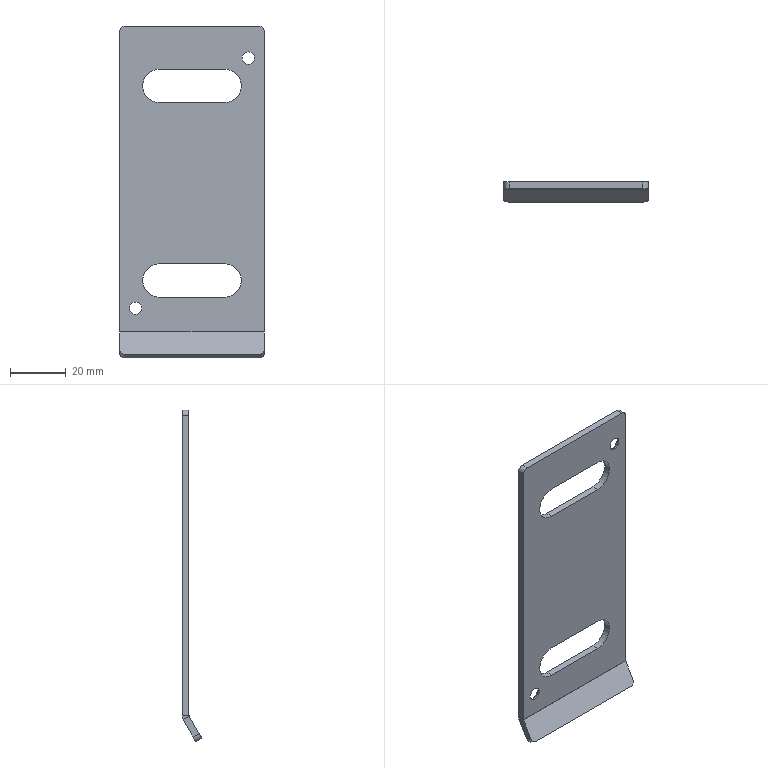Part | STEP file | touch screen guide plate | 1 solid | 34 faces | box 52 x 7.165 x 119.33 mm | volume 13457 mm3 | plane 16 | cylinder 14 | cone 4 | commonest cylinder face diameters 4 x4 4.5 x4 12 x4 0.2 x1 5.2 x1